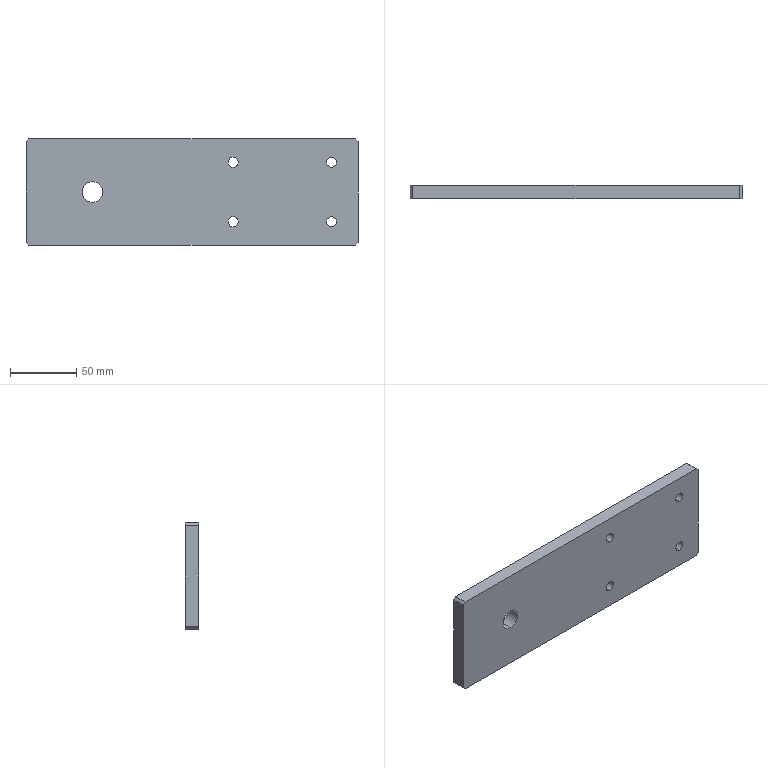Part | SolidWorks | features ICE 1, SplitBody 1 | 1 solid | 20 faces | box 250 x 10 x 80 mm | volume 196266 mm3 | cylinder 10 | plane 10 | commonest cylinder face diameters 7.5 x8 15.5 x2
STEP:
#1=CARTESIAN_POINT('',(-500.,-53.,-267.75));
#2=VERTEX_POINT('',#1);
#3=CARTESIAN_POINT('',(-500.,-53.,-252.25));
#4=VERTEX_POINT('',#3);
#5=CARTESIAN_POINT('',(-500.,-53.,-260.));
#6=DIRECTION('',(0.,-1.,0.));
#7=DIRECTION('',(0.,0.,-1.));
#8=AXIS2_PLACEMENT_3D('',#5,#6,#7);
#9=CIRCLE('',#8,7.75);
#10=EDGE_CURVE('',#2,#4,#9,.T.);
#11=ORIENTED_EDGE('',*,*,#10,.F.);
#12=CARTESIAN_POINT('',(-500.,-63.,-267.75));
#13=VERTEX_POINT('',#12);
#14=CARTESIAN_POINT('',(-500.,-58.,-267.75));
#15=DIRECTION('',(0.,-1.,0.));
#16=VECTOR('',#15,1000.);
#17=LINE('',#14,#16);
#18=EDGE_CURVE('',#2,#13,#17,.T.);
#19=ORIENTED_EDGE('',*,*,#18,.T.);
#20=CARTESIAN_POINT('',(-500.,-63.,-252.25));
#21=VERTEX_POINT('',#20);
#22=CARTESIAN_POINT('',(-500.,-63.,-260.));
#23=DIRECTION('',(0.,1.,0.));
#24=DIRECTION('',(0.,0.,1.));
#25=AXIS2_PLACEMENT_3D('',#22,#23,#24);
#26=CIRCLE('',#25,7.75);
#27=EDGE_CURVE('',#21,#13,#26,.T.);
#28=ORIENTED_EDGE('',*,*,#27,.F.);
#29=CARTESIAN_POINT('',(-500.,-58.,-252.25));
#30=DIRECTION('',(0.,-1.,0.));
#31=VECTOR('',#30,1000.);
#32=LINE('',#29,#31);
#33=EDGE_CURVE('',#4,#21,#32,.T.);
#34=ORIENTED_EDGE('',*,*,#33,.F.);
#35=EDGE_LOOP('',(#11,#19,#28,#34));
#36=FACE_OUTER_BOUND('',#35,.T.);
#37=CARTESIAN_POINT('',(-500.,-58.,-260.));
#38=DIRECTION('',(0.,-1.,0.));
#39=DIRECTION('',(0.,0.,1.));
#40=AXIS2_PLACEMENT_3D('',#37,#38,#39);
#41=CYLINDRICAL_SURFACE('',#40,7.75);
#42=ADVANCED_FACE('',(#36),#41,.F.);
#43=CARTESIAN_POINT('',(-394.,-53.,-241.35));
#44=VERTEX_POINT('',#43);
#45=CARTESIAN_POINT('',(-394.,-53.,-233.85));
#46=VERTEX_POINT('',#45);
#47=CARTESIAN_POINT('',(-394.,-53.,-237.6));
#48=DIRECTION('',(0.,-1.,0.));
#49=DIRECTION('',(0.,0.,-1.));
#50=AXIS2_PLACEMENT_3D('',#47,#48,#49);
#51=CIRCLE('',#50,3.75);
#52=EDGE_CURVE('',#44,#46,#51,.T.);
#53=ORIENTED_EDGE('',*,*,#52,.F.);
#54=CARTESIAN_POINT('',(-394.,-63.,-241.35));
#55=VERTEX_POINT('',#54);
#56=CARTESIAN_POINT('',(-394.,-58.,-241.35));
#57=DIRECTION('',(0.,-1.,0.));
#58=VECTOR('',#57,1000.);
#59=LINE('',#56,#58);
#60=EDGE_CURVE('',#44,#55,#59,.T.);
#61=ORIENTED_EDGE('',*,*,#60,.T.);
#62=CARTESIAN_POINT('',(-394.,-63.,-233.85));
#63=VERTEX_POINT('',#62);
#64=CARTESIAN_POINT('',(-394.,-63.,-237.6));
#65=DIRECTION('',(0.,1.,0.));
#66=DIRECTION('',(0.,0.,1.));
#67=AXIS2_PLACEMENT_3D('',#64,#65,#66);
#68=CIRCLE('',#67,3.75);
#69=EDGE_CURVE('',#63,#55,#68,.T.);
#70=ORIENTED_EDGE('',*,*,#69,.F.);
#71=CARTESIAN_POINT('',(-394.,-58.,-233.85));
#72=DIRECTION('',(0.,-1.,0.));
#73=VECTOR('',#72,1000.);
#74=LINE('',#71,#73);
#75=EDGE_CURVE('',#46,#63,#74,.T.);
#76=ORIENTED_EDGE('',*,*,#75,.F.);
#77=EDGE_LOOP('',(#53,#61,#70,#76));
#78=FACE_OUTER_BOUND('',#77,.T.);
#79=CARTESIAN_POINT('',(-394.,-58.,-237.6));
#80=DIRECTION('',(0.,-1.,0.));
#81=DIRECTION('',(0.,0.,1.));
#82=AXIS2_PLACEMENT_3D('',#79,#80,#81);
#83=CYLINDRICAL_SURFACE('',#82,3.75);
#84=ADVANCED_FACE('',(#78),#83,.F.);
#85=CARTESIAN_POINT('',(-320.,-53.,-241.35));
#86=VERTEX_POINT('',#85);
#87=CARTESIAN_POINT('',(-320.,-53.,-233.85));
#88=VERTEX_POINT('',#87);
#89=CARTESIAN_POINT('',(-320.,-53.,-237.6));
#90=DIRECTION('',(0.,-1.,0.));
#91=DIRECTION('',(0.,0.,-1.));
#92=AXIS2_PLACEMENT_3D('',#89,#90,#91);
#93=CIRCLE('',#92,3.75);
#94=EDGE_CURVE('',#86,#88,#93,.T.);
#95=ORIENTED_EDGE('',*,*,#94,.F.);
#96=CARTESIAN_POINT('',(-320.,-63.,-241.35));
#97=VERTEX_POINT('',#96);
#98=CARTESIAN_POINT('',(-320.,-58.,-241.35));
#99=DIRECTION('',(0.,-1.,0.));
#100=VECTOR('',#99,1000.);
#101=LINE('',#98,#100);
#102=EDGE_CURVE('',#86,#97,#101,.T.);
#103=ORIENTED_EDGE('',*,*,#102,.T.);
#104=CARTESIAN_POINT('',(-320.,-63.,-233.85));
#105=VERTEX_POINT('',#104);
#106=CARTESIAN_POINT('',(-320.,-63.,-237.6));
#107=DIRECTION('',(0.,1.,0.));
#108=DIRECTION('',(0.,0.,1.));
#109=AXIS2_PLACEMENT_3D('',#106,#107,#108);
#110=CIRCLE('',#109,3.75);
#111=EDGE_CURVE('',#105,#97,#110,.T.);
#112=ORIENTED_EDGE('',*,*,#111,.F.);
#113=CARTESIAN_POINT('',(-320.,-58.,-233.85));
#114=DIRECTION('',(0.,-1.,0.));
#115=VECTOR('',#114,1000.);
#116=LINE('',#113,#115);
#117=EDGE_CURVE('',#88,#105,#116,.T.);
#118=ORIENTED_EDGE('',*,*,#117,.F.);
#119=EDGE_LOOP('',(#95,#103,#112,#118));
#120=FACE_OUTER_BOUND('',#119,.T.);
#121=CARTESIAN_POINT('',(-320.,-58.,-237.6));
#122=DIRECTION('',(0.,-1.,0.));
#123=DIRECTION('',(0.,0.,1.));
#124=AXIS2_PLACEMENT_3D('',#121,#122,#123);
#125=CYLINDRICAL_SURFACE('',#124,3.75);
#126=ADVANCED_FACE('',(#120),#125,.F.);
#127=CARTESIAN_POINT('',(-320.,-53.,-286.15));
#128=VERTEX_POINT('',#127);
#129=CARTESIAN_POINT('',(-320.,-53.,-278.65));
#130=VERTEX_POINT('',#129);
#131=CARTESIAN_POINT('',(-320.,-53.,-282.4));
#132=DIRECTION('',(0.,-1.,0.));
#133=DIRECTION('',(0.,0.,-1.));
#134=AXIS2_PLACEMENT_3D('',#131,#132,#133);
#135=CIRCLE('',#134,3.75);
#136=EDGE_CURVE('',#128,#130,#135,.T.);
#137=ORIENTED_EDGE('',*,*,#136,.F.);
#138=CARTESIAN_POINT('',(-320.,-63.,-286.15));
#139=VERTEX_POINT('',#138);
#140=CARTESIAN_POINT('',(-320.,-58.,-286.15));
#141=DIRECTION('',(0.,-1.,0.));
#142=VECTOR('',#141,1000.);
#143=LINE('',#140,#142);
#144=EDGE_CURVE('',#128,#139,#143,.T.);
#145=ORIENTED_EDGE('',*,*,#144,.T.);
#146=CARTESIAN_POINT('',(-320.,-63.,-278.65));
#147=VERTEX_POINT('',#146);
#148=CARTESIAN_POINT('',(-320.,-63.,-282.4));
#149=DIRECTION('',(0.,1.,0.));
#150=DIRECTION('',(0.,0.,1.));
#151=AXIS2_PLACEMENT_3D('',#148,#149,#150);
#152=CIRCLE('',#151,3.75);
#153=EDGE_CURVE('',#147,#139,#152,.T.);
#154=ORIENTED_EDGE('',*,*,#153,.F.);
#155=CARTESIAN_POINT('',(-320.,-58.,-278.65));
#156=DIRECTION('',(0.,-1.,0.));
#157=VECTOR('',#156,1000.);
#158=LINE('',#155,#157);
#159=EDGE_CURVE('',#130,#147,#158,.T.);
#160=ORIENTED_EDGE('',*,*,#159,.F.);
#161=EDGE_LOOP('',(#137,#145,#154,#160));
#162=FACE_OUTER_BOUND('',#161,.T.);
#163=CARTESIAN_POINT('',(-320.,-58.,-282.4));
#164=DIRECTION('',(0.,-1.,0.));
#165=DIRECTION('',(0.,0.,1.));
#166=AXIS2_PLACEMENT_3D('',#163,#164,#165);
#167=CYLINDRICAL_SURFACE('',#166,3.75);
#168=ADVANCED_FACE('',(#162),#167,.F.);
#169=CARTESIAN_POINT('',(-394.,-53.,-286.15));
#170=VERTEX_POINT('',#169);
#171=CARTESIAN_POINT('',(-394.,-53.,-278.65));
#172=VERTEX_POINT('',#171);
#173=CARTESIAN_POINT('',(-394.,-53.,-282.4));
#174=DIRECTION('',(0.,-1.,0.));
#175=DIRECTION('',(0.,0.,-1.));
#176=AXIS2_PLACEMENT_3D('',#173,#174,#175);
#177=CIRCLE('',#176,3.75);
#178=EDGE_CURVE('',#170,#172,#177,.T.);
#179=ORIENTED_EDGE('',*,*,#178,.F.);
#180=CARTESIAN_POINT('',(-394.,-63.,-286.15));
#181=VERTEX_POINT('',#180);
#182=CARTESIAN_POINT('',(-394.,-58.,-286.15));
#183=DIRECTION('',(0.,-1.,0.));
#184=VECTOR('',#183,1000.);
#185=LINE('',#182,#184);
#186=EDGE_CURVE('',#170,#181,#185,.T.);
#187=ORIENTED_EDGE('',*,*,#186,.T.);
#188=CARTESIAN_POINT('',(-394.,-63.,-278.65));
#189=VERTEX_POINT('',#188);
#190=CARTESIAN_POINT('',(-394.,-63.,-282.4));
#191=DIRECTION('',(0.,1.,0.));
#192=DIRECTION('',(0.,0.,1.));
#193=AXIS2_PLACEMENT_3D('',#190,#191,#192);
#194=CIRCLE('',#193,3.75);
#195=EDGE_CURVE('',#189,#181,#194,.T.);
#196=ORIENTED_EDGE('',*,*,#195,.F.);
#197=CARTESIAN_POINT('',(-394.,-58.,-278.65));
#198=DIRECTION('',(0.,-1.,0.));
#199=VECTOR('',#198,1000.);
#200=LINE('',#197,#199);
#201=EDGE_CURVE('',#172,#189,#200,.T.);
#202=ORIENTED_EDGE('',*,*,#201,.F.);
#203=EDGE_LOOP('',(#179,#187,#196,#202));
#204=FACE_OUTER_BOUND('',#203,.T.);
#205=CARTESIAN_POINT('',(-394.,-58.,-282.4));
#206=DIRECTION('',(0.,-1.,0.));
#207=DIRECTION('',(0.,0.,1.));
#208=AXIS2_PLACEMENT_3D('',#205,#206,#207);
#209=CYLINDRICAL_SURFACE('',#208,3.75);
#210=ADVANCED_FACE('',(#204),#209,.F.);
#211=CARTESIAN_POINT('',(-550.,-53.,-298.));
#212=VERTEX_POINT('',#211);
#213=CARTESIAN_POINT('',(-550.,-53.,-222.));
#214=VERTEX_POINT('',#213);
#215=CARTESIAN_POINT('',(-550.,-53.,-300.));
#216=DIRECTION('',(0.,0.,1.));
#217=VECTOR('',#216,1000.);
#218=LINE('',#215,#217);
#219=EDGE_CURVE('',#212,#214,#218,.T.);
#220=ORIENTED_EDGE('',*,*,#219,.F.);
#221=CARTESIAN_POINT('',(-550.,-63.,-298.));
#222=VERTEX_POINT('',#221);
#223=CARTESIAN_POINT('',(-550.,-63.,-298.));
#224=DIRECTION('',(0.,1.,0.));
#225=VECTOR('',#224,1000.);
#226=LINE('',#223,#225);
#227=EDGE_CURVE('',#222,#212,#226,.T.);
#228=ORIENTED_EDGE('',*,*,#227,.F.);
#229=CARTESIAN_POINT('',(-550.,-63.,-222.));
#230=VERTEX_POINT('',#229);
#231=CARTESIAN_POINT('',(-550.,-63.,-300.));
#232=DIRECTION('',(0.,0.,1.));
#233=VECTOR('',#232,1000.);
#234=LINE('',#231,#233);
#235=EDGE_CURVE('',#222,#230,#234,.T.);
#236=ORIENTED_EDGE('',*,*,#235,.T.);
#237=CARTESIAN_POINT('',(-550.,-63.,-222.));
#238=DIRECTION('',(0.,-1.,0.));
#239=VECTOR('',#238,1000.);
#240=LINE('',#237,#239);
#241=EDGE_CURVE('',#214,#230,#240,.T.);
#242=ORIENTED_EDGE('',*,*,#241,.F.);
#243=EDGE_LOOP('',(#220,#228,#236,#242));
#244=FACE_OUTER_BOUND('',#243,.T.);
#245=CARTESIAN_POINT('',(-550.,-63.,-300.));
#246=DIRECTION('',(1.,0.,0.));
#247=DIRECTION('',(0.,1.,0.));
#248=AXIS2_PLACEMENT_3D('',#245,#246,#247);
#249=PLANE('',#248);
#250=ADVANCED_FACE('',(#244),#249,.F.);
#251=CARTESIAN_POINT('',(-548.,-53.,-220.));
#252=VERTEX_POINT('',#251);
#253=CARTESIAN_POINT('',(-302.,-53.,-220.));
#254=VERTEX_POINT('',#253);
#255=CARTESIAN_POINT('',(-550.,-53.,-220.));
#256=DIRECTION('',(1.,0.,0.));
#257=VECTOR('',#256,1000.);
#258=LINE('',#255,#257);
#259=EDGE_CURVE('',#252,#254,#258,.T.);
#260=ORIENTED_EDGE('',*,*,#259,.F.);
#261=CARTESIAN_POINT('',(-548.,-63.,-220.));
#262=VERTEX_POINT('',#261);
#263=CARTESIAN_POINT('',(-548.,-63.,-220.));
#264=DIRECTION('',(0.,1.,0.));
#265=VECTOR('',#264,1000.);
#266=LINE('',#263,#265);
#267=EDGE_CURVE('',#262,#252,#266,.T.);
#268=ORIENTED_EDGE('',*,*,#267,.F.);
#269=CARTESIAN_POINT('',(-302.,-63.,-220.));
#270=VERTEX_POINT('',#269);
#271=CARTESIAN_POINT('',(-550.,-63.,-220.));
#272=DIRECTION('',(1.,0.,0.));
#273=VECTOR('',#272,1000.);
#274=LINE('',#271,#273);
#275=EDGE_CURVE('',#262,#270,#274,.T.);
#276=ORIENTED_EDGE('',*,*,#275,.T.);
#277=CARTESIAN_POINT('',(-302.,-63.,-220.));
#278=DIRECTION('',(0.,-1.,0.));
#279=VECTOR('',#278,1000.);
#280=LINE('',#277,#279);
#281=EDGE_CURVE('',#254,#270,#280,.T.);
#282=ORIENTED_EDGE('',*,*,#281,.F.);
#283=EDGE_LOOP('',(#260,#268,#276,#282));
#284=FACE_OUTER_BOUND('',#283,.T.);
#285=CARTESIAN_POINT('',(-550.,-63.,-220.));
#286=DIRECTION('',(0.,0.,-1.));
#287=DIRECTION('',(0.,-1.,0.));
#288=AXIS2_PLACEMENT_3D('',#285,#286,#287);
#289=PLANE('',#288);
#290=ADVANCED_FACE('',(#284),#289,.F.);
#291=CARTESIAN_POINT('',(-300.,-63.,-222.));
#292=VERTEX_POINT('',#291);
#293=CARTESIAN_POINT('',(-300.,-63.,-298.));
#294=VERTEX_POINT('',#293);
#295=CARTESIAN_POINT('',(-300.,-63.,-300.));
#296=DIRECTION('',(0.,0.,-1.));
#297=VECTOR('',#296,1000.);
#298=LINE('',#295,#297);
#299=EDGE_CURVE('',#292,#294,#298,.T.);
#300=ORIENTED_EDGE('',*,*,#299,.T.);
#301=CARTESIAN_POINT('',(-300.,-53.,-298.));
#302=VERTEX_POINT('',#301);
#303=CARTESIAN_POINT('',(-300.,-63.,-298.));
#304=DIRECTION('',(0.,-1.,0.));
#305=VECTOR('',#304,1000.);
#306=LINE('',#303,#305);
#307=EDGE_CURVE('',#302,#294,#306,.T.);
#308=ORIENTED_EDGE('',*,*,#307,.F.);
#309=CARTESIAN_POINT('',(-300.,-53.,-222.));
#310=VERTEX_POINT('',#309);
#311=CARTESIAN_POINT('',(-300.,-53.,-300.));
#312=DIRECTION('',(0.,0.,-1.));
#313=VECTOR('',#312,1000.);
#314=LINE('',#311,#313);
#315=EDGE_CURVE('',#310,#302,#314,.T.);
#316=ORIENTED_EDGE('',*,*,#315,.F.);
#317=CARTESIAN_POINT('',(-300.,-63.,-222.));
#318=DIRECTION('',(0.,1.,0.));
#319=VECTOR('',#318,1000.);
#320=LINE('',#317,#319);
#321=EDGE_CURVE('',#292,#310,#320,.T.);
#322=ORIENTED_EDGE('',*,*,#321,.F.);
#323=EDGE_LOOP('',(#300,#308,#316,#322));
#324=FACE_OUTER_BOUND('',#323,.T.);
#325=CARTESIAN_POINT('',(-300.,-63.,-300.));
#326=DIRECTION('',(-1.,0.,0.));
#327=DIRECTION('',(0.,-1.,0.));
#328=AXIS2_PLACEMENT_3D('',#325,#326,#327);
#329=PLANE('',#328);
#330=ADVANCED_FACE('',(#324),#329,.F.);
#331=CARTESIAN_POINT('',(-302.,-63.,-300.));
#332=VERTEX_POINT('',#331);
#333=CARTESIAN_POINT('',(-548.,-63.,-300.));
#334=VERTEX_POINT('',#333);
#335=CARTESIAN_POINT('',(-550.,-63.,-300.));
#336=DIRECTION('',(-1.,0.,0.));
#337=VECTOR('',#336,1000.);
#338=LINE('',#335,#337);
#339=EDGE_CURVE('',#332,#334,#338,.T.);
#340=ORIENTED_EDGE('',*,*,#339,.T.);
#341=CARTESIAN_POINT('',(-548.,-53.,-300.));
#342=VERTEX_POINT('',#341);
#343=CARTESIAN_POINT('',(-548.,-63.,-300.));
#344=DIRECTION('',(0.,-1.,0.));
#345=VECTOR('',#344,1000.);
#346=LINE('',#343,#345);
#347=EDGE_CURVE('',#342,#334,#346,.T.);
#348=ORIENTED_EDGE('',*,*,#347,.F.);
#349=CARTESIAN_POINT('',(-302.,-53.,-300.));
#350=VERTEX_POINT('',#349);
#351=CARTESIAN_POINT('',(-550.,-53.,-300.));
#352=DIRECTION('',(-1.,0.,0.));
#353=VECTOR('',#352,1000.);
#354=LINE('',#351,#353);
#355=EDGE_CURVE('',#350,#342,#354,.T.);
#356=ORIENTED_EDGE('',*,*,#355,.F.);
#357=CARTESIAN_POINT('',(-302.,-63.,-300.));
#358=DIRECTION('',(0.,1.,0.));
#359=VECTOR('',#358,1000.);
#360=LINE('',#357,#359);
#361=EDGE_CURVE('',#332,#350,#360,.T.);
#362=ORIENTED_EDGE('',*,*,#361,.F.);
#363=EDGE_LOOP('',(#340,#348,#356,#362));
#364=FACE_OUTER_BOUND('',#363,.T.);
#365=CARTESIAN_POINT('',(-550.,-63.,-300.));
#366=DIRECTION('',(0.,0.,1.));
#367=DIRECTION('',(0.,1.,0.));
#368=AXIS2_PLACEMENT_3D('',#365,#366,#367);
#369=PLANE('',#368);
#370=ADVANCED_FACE('',(#364),#369,.F.);
#371=ORIENTED_EDGE('',*,*,#27,.T.);
#372=CARTESIAN_POINT('',(-500.,-63.,-260.));
#373=DIRECTION('',(0.,1.,0.));
#374=DIRECTION('',(0.,0.,1.));
#375=AXIS2_PLACEMENT_3D('',#372,#373,#374);
#376=CIRCLE('',#375,7.75);
#377=EDGE_CURVE('',#13,#21,#376,.T.);
#378=ORIENTED_EDGE('',*,*,#377,.T.);
#379=EDGE_LOOP('',(#371,#378));
#380=FACE_BOUND('',#379,.T.);
#381=ORIENTED_EDGE('',*,*,#69,.T.);
#382=CARTESIAN_POINT('',(-394.,-63.,-237.6));
#383=DIRECTION('',(0.,1.,0.));
#384=DIRECTION('',(0.,0.,1.));
#385=AXIS2_PLACEMENT_3D('',#382,#383,#384);
#386=CIRCLE('',#385,3.75);
#387=EDGE_CURVE('',#55,#63,#386,.T.);
#388=ORIENTED_EDGE('',*,*,#387,.T.);
#389=EDGE_LOOP('',(#381,#388));
#390=FACE_BOUND('',#389,.T.);
#391=ORIENTED_EDGE('',*,*,#111,.T.);
#392=CARTESIAN_POINT('',(-320.,-63.,-237.6));
#393=DIRECTION('',(0.,1.,0.));
#394=DIRECTION('',(0.,0.,1.));
#395=AXIS2_PLACEMENT_3D('',#392,#393,#394);
#396=CIRCLE('',#395,3.75);
#397=EDGE_CURVE('',#97,#105,#396,.T.);
#398=ORIENTED_EDGE('',*,*,#397,.T.);
#399=EDGE_LOOP('',(#391,#398));
#400=FACE_BOUND('',#399,.T.);
#401=ORIENTED_EDGE('',*,*,#153,.T.);
#402=CARTESIAN_POINT('',(-320.,-63.,-282.4));
#403=DIRECTION('',(0.,1.,0.));
#404=DIRECTION('',(0.,0.,1.));
#405=AXIS2_PLACEMENT_3D('',#402,#403,#404);
#406=CIRCLE('',#405,3.75);
#407=EDGE_CURVE('',#139,#147,#406,.T.);
#408=ORIENTED_EDGE('',*,*,#407,.T.);
#409=EDGE_LOOP('',(#401,#408));
#410=FACE_BOUND('',#409,.T.);
#411=ORIENTED_EDGE('',*,*,#195,.T.);
#412=CARTESIAN_POINT('',(-394.,-63.,-282.4));
#413=DIRECTION('',(0.,1.,0.));
#414=DIRECTION('',(0.,0.,1.));
#415=AXIS2_PLACEMENT_3D('',#412,#413,#414);
#416=CIRCLE('',#415,3.75);
#417=EDGE_CURVE('',#181,#189,#416,.T.);
#418=ORIENTED_EDGE('',*,*,#417,.T.);
#419=EDGE_LOOP('',(#411,#418));
#420=FACE_BOUND('',#419,.T.);
#421=ORIENTED_EDGE('',*,*,#275,.F.);
#422=CARTESIAN_POINT('',(-164.,-63.,164.));
#423=DIRECTION('',(0.7071,0.,0.7071));
#424=VECTOR('',#423,1000.);
#425=LINE('',#422,#424);
#426=EDGE_CURVE('',#230,#262,#425,.T.);
#427=ORIENTED_EDGE('',*,*,#426,.F.);
#428=ORIENTED_EDGE('',*,*,#235,.F.);
#429=CARTESIAN_POINT('',(-424.,-63.,-424.));
#430=DIRECTION('',(-0.7071,0.,0.7071));
#431=VECTOR('',#430,1000.);
#432=LINE('',#429,#431);
#433=EDGE_CURVE('',#334,#222,#432,.T.);
#434=ORIENTED_EDGE('',*,*,#433,.F.);
#435=ORIENTED_EDGE('',*,*,#339,.F.);
#436=CARTESIAN_POINT('',(-1.,-63.,1.));
#437=DIRECTION('',(-0.7071,0.,-0.7071));
#438=VECTOR('',#437,1000.);
#439=LINE('',#436,#438);
#440=EDGE_CURVE('',#294,#332,#439,.T.);
#441=ORIENTED_EDGE('',*,*,#440,.F.);
#442=ORIENTED_EDGE('',*,*,#299,.F.);
#443=CARTESIAN_POINT('',(-261.,-63.,-261.));
#444=DIRECTION('',(0.7071,0.,-0.7071));
#445=VECTOR('',#444,1000.);
#446=LINE('',#443,#445);
#447=EDGE_CURVE('',#270,#292,#446,.T.);
#448=ORIENTED_EDGE('',*,*,#447,.F.);
#449=EDGE_LOOP('',(#421,#427,#428,#434,#435,#441,#442,#448));
#450=FACE_OUTER_BOUND('',#449,.T.);
#451=CARTESIAN_POINT('',(0.,-63.,0.));
#452=DIRECTION('',(0.,-1.,0.));
#453=DIRECTION('',(0.,0.,1.));
#454=AXIS2_PLACEMENT_3D('',#451,#452,#453);
#455=PLANE('',#454);
#456=ADVANCED_FACE('',(#380,#390,#400,#410,#420,#450),#455,.T.);
#457=CARTESIAN_POINT('',(-394.,-53.,-237.6));
#458=DIRECTION('',(0.,-1.,0.));
#459=DIRECTION('',(0.,0.,-1.));
#460=AXIS2_PLACEMENT_3D('',#457,#458,#459);
#461=CIRCLE('',#460,3.75);
#462=EDGE_CURVE('',#46,#44,#461,.T.);
#463=ORIENTED_EDGE('',*,*,#462,.T.);
#464=ORIENTED_EDGE('',*,*,#52,.T.);
#465=EDGE_LOOP('',(#463,#464));
#466=FACE_BOUND('',#465,.T.);
#467=CARTESIAN_POINT('',(-394.,-53.,-282.4));
#468=DIRECTION('',(0.,-1.,0.));
#469=DIRECTION('',(0.,0.,-1.));
#470=AXIS2_PLACEMENT_3D('',#467,#468,#469);
#471=CIRCLE('',#470,3.75);
#472=EDGE_CURVE('',#172,#170,#471,.T.);
#473=ORIENTED_EDGE('',*,*,#472,.T.);
#474=ORIENTED_EDGE('',*,*,#178,.T.);
#475=EDGE_LOOP('',(#473,#474));
#476=FACE_BOUND('',#475,.T.);
#477=CARTESIAN_POINT('',(-320.,-53.,-237.6));
#478=DIRECTION('',(0.,-1.,0.));
#479=DIRECTION('',(0.,0.,-1.));
#480=AXIS2_PLACEMENT_3D('',#477,#478,#479);
#481=CIRCLE('',#480,3.75);
#482=EDGE_CURVE('',#88,#86,#481,.T.);
#483=ORIENTED_EDGE('',*,*,#482,.T.);
#484=ORIENTED_EDGE('',*,*,#94,.T.);
#485=EDGE_LOOP('',(#483,#484));
#486=FACE_BOUND('',#485,.T.);
#487=CARTESIAN_POINT('',(-320.,-53.,-282.4));
#488=DIRECTION('',(0.,-1.,0.));
#489=DIRECTION('',(0.,0.,-1.));
#490=AXIS2_PLACEMENT_3D('',#487,#488,#489);
#491=CIRCLE('',#490,3.75);
#492=EDGE_CURVE('',#130,#128,#491,.T.);
#493=ORIENTED_EDGE('',*,*,#492,.T.);
#494=ORIENTED_EDGE('',*,*,#136,.T.);
#495=EDGE_LOOP('',(#493,#494));
#496=FACE_BOUND('',#495,.T.);
#497=CARTESIAN_POINT('',(-500.,-53.,-260.));
#498=DIRECTION('',(0.,-1.,0.));
#499=DIRECTION('',(0.,0.,-1.));
#500=AXIS2_PLACEMENT_3D('',#497,#498,#499);
#501=CIRCLE('',#500,7.75);
#502=EDGE_CURVE('',#4,#2,#501,.T.);
#503=ORIENTED_EDGE('',*,*,#502,.T.);
#504=ORIENTED_EDGE('',*,*,#10,.T.);
#505=EDGE_LOOP('',(#503,#504));
#506=FACE_BOUND('',#505,.T.);
#507=ORIENTED_EDGE('',*,*,#315,.T.);
#508=CARTESIAN_POINT('',(-302.,-53.,-300.));
#509=DIRECTION('',(0.7071,0.,0.7071));
#510=VECTOR('',#509,1000.);
#511=LINE('',#508,#510);
#512=EDGE_CURVE('',#350,#302,#511,.T.);
#513=ORIENTED_EDGE('',*,*,#512,.F.);
#514=ORIENTED_EDGE('',*,*,#355,.T.);
#515=CARTESIAN_POINT('',(-550.,-53.,-298.));
#516=DIRECTION('',(0.7071,0.,-0.7071));
#517=VECTOR('',#516,1000.);
#518=LINE('',#515,#517);
#519=EDGE_CURVE('',#212,#342,#518,.T.);
#520=ORIENTED_EDGE('',*,*,#519,.F.);
#521=ORIENTED_EDGE('',*,*,#219,.T.);
#522=CARTESIAN_POINT('',(-548.,-53.,-220.));
#523=DIRECTION('',(-0.7071,0.,-0.7071));
#524=VECTOR('',#523,1000.);
#525=LINE('',#522,#524);
#526=EDGE_CURVE('',#252,#214,#525,.T.);
#527=ORIENTED_EDGE('',*,*,#526,.F.);
#528=ORIENTED_EDGE('',*,*,#259,.T.);
#529=CARTESIAN_POINT('',(-300.,-53.,-222.));
#530=DIRECTION('',(-0.7071,0.,0.7071));
#531=VECTOR('',#530,1000.);
#532=LINE('',#529,#531);
#533=EDGE_CURVE('',#310,#254,#532,.T.);
#534=ORIENTED_EDGE('',*,*,#533,.F.);
#535=EDGE_LOOP('',(#507,#513,#514,#520,#521,#527,#528,#534));
#536=FACE_OUTER_BOUND('',#535,.T.);
#537=CARTESIAN_POINT('',(0.,-53.,0.));
#538=DIRECTION('',(0.,-1.,0.));
#539=DIRECTION('',(0.,0.,1.));
#540=AXIS2_PLACEMENT_3D('',#537,#538,#539);
#541=PLANE('',#540);
#542=ADVANCED_FACE('',(#466,#476,#486,#496,#506,#536),#541,.F.);
#543=ORIENTED_EDGE('',*,*,#186,.F.);
#544=ORIENTED_EDGE('',*,*,#472,.F.);
#545=ORIENTED_EDGE('',*,*,#201,.T.);
#546=ORIENTED_EDGE('',*,*,#417,.F.);
#547=EDGE_LOOP('',(#543,#544,#545,#546));
#548=FACE_OUTER_BOUND('',#547,.T.);
#549=CARTESIAN_POINT('',(-394.,-58.,-282.4));
#550=DIRECTION('',(0.,-1.,0.));
#551=DIRECTION('',(0.,0.,1.));
#552=AXIS2_PLACEMENT_3D('',#549,#550,#551);
#553=CYLINDRICAL_SURFACE('',#552,3.75);
#554=ADVANCED_FACE('',(#548),#553,.F.);
#555=ORIENTED_EDGE('',*,*,#144,.F.);
#556=ORIENTED_EDGE('',*,*,#492,.F.);
#557=ORIENTED_EDGE('',*,*,#159,.T.);
#558=ORIENTED_EDGE('',*,*,#407,.F.);
#559=EDGE_LOOP('',(#555,#556,#557,#558));
#560=FACE_OUTER_BOUND('',#559,.T.);
#561=CARTESIAN_POINT('',(-320.,-58.,-282.4));
#562=DIRECTION('',(0.,-1.,0.));
#563=DIRECTION('',(0.,0.,1.));
#564=AXIS2_PLACEMENT_3D('',#561,#562,#563);
#565=CYLINDRICAL_SURFACE('',#564,3.75);
#566=ADVANCED_FACE('',(#560),#565,.F.);
#567=ORIENTED_EDGE('',*,*,#102,.F.);
#568=ORIENTED_EDGE('',*,*,#482,.F.);
#569=ORIENTED_EDGE('',*,*,#117,.T.);
#570=ORIENTED_EDGE('',*,*,#397,.F.);
#571=EDGE_LOOP('',(#567,#568,#569,#570));
#572=FACE_OUTER_BOUND('',#571,.T.);
#573=CARTESIAN_POINT('',(-320.,-58.,-237.6));
#574=DIRECTION('',(0.,-1.,0.));
#575=DIRECTION('',(0.,0.,1.));
#576=AXIS2_PLACEMENT_3D('',#573,#574,#575);
#577=CYLINDRICAL_SURFACE('',#576,3.75);
#578=ADVANCED_FACE('',(#572),#577,.F.);
#579=ORIENTED_EDGE('',*,*,#60,.F.);
#580=ORIENTED_EDGE('',*,*,#462,.F.);
#581=ORIENTED_EDGE('',*,*,#75,.T.);
#582=ORIENTED_EDGE('',*,*,#387,.F.);
#583=EDGE_LOOP('',(#579,#580,#581,#582));
#584=FACE_OUTER_BOUND('',#583,.T.);
#585=CARTESIAN_POINT('',(-394.,-58.,-237.6));
#586=DIRECTION('',(0.,-1.,0.));
#587=DIRECTION('',(0.,0.,1.));
#588=AXIS2_PLACEMENT_3D('',#585,#586,#587);
#589=CYLINDRICAL_SURFACE('',#588,3.75);
#590=ADVANCED_FACE('',(#584),#589,.F.);
#591=ORIENTED_EDGE('',*,*,#447,.T.);
#592=ORIENTED_EDGE('',*,*,#321,.T.);
#593=ORIENTED_EDGE('',*,*,#533,.T.);
#594=ORIENTED_EDGE('',*,*,#281,.T.);
#595=EDGE_LOOP('',(#591,#592,#593,#594));
#596=FACE_OUTER_BOUND('',#595,.T.);
#597=CARTESIAN_POINT('',(-300.,-63.,-222.));
#598=DIRECTION('',(-0.7071,0.,-0.7071));
#599=DIRECTION('',(0.,1.,0.));
#600=AXIS2_PLACEMENT_3D('',#597,#598,#599);
#601=PLANE('',#600);
#602=ADVANCED_FACE('',(#596),#601,.F.);
#603=ORIENTED_EDGE('',*,*,#440,.T.);
#604=ORIENTED_EDGE('',*,*,#361,.T.);
#605=ORIENTED_EDGE('',*,*,#512,.T.);
#606=ORIENTED_EDGE('',*,*,#307,.T.);
#607=EDGE_LOOP('',(#603,#604,#605,#606));
#608=FACE_OUTER_BOUND('',#607,.T.);
#609=CARTESIAN_POINT('',(-302.,-63.,-300.));
#610=DIRECTION('',(-0.7071,0.,0.7071));
#611=DIRECTION('',(0.,1.,0.));
#612=AXIS2_PLACEMENT_3D('',#609,#610,#611);
#613=PLANE('',#612);
#614=ADVANCED_FACE('',(#608),#613,.F.);
#615=ORIENTED_EDGE('',*,*,#426,.T.);
#616=ORIENTED_EDGE('',*,*,#267,.T.);
#617=ORIENTED_EDGE('',*,*,#526,.T.);
#618=ORIENTED_EDGE('',*,*,#241,.T.);
#619=EDGE_LOOP('',(#615,#616,#617,#618));
#620=FACE_OUTER_BOUND('',#619,.T.);
#621=CARTESIAN_POINT('',(-548.,-63.,-220.));
#622=DIRECTION('',(0.7071,0.,-0.7071));
#623=DIRECTION('',(0.,1.,0.));
#624=AXIS2_PLACEMENT_3D('',#621,#622,#623);
#625=PLANE('',#624);
#626=ADVANCED_FACE('',(#620),#625,.F.);
#627=ORIENTED_EDGE('',*,*,#433,.T.);
#628=ORIENTED_EDGE('',*,*,#227,.T.);
#629=ORIENTED_EDGE('',*,*,#519,.T.);
#630=ORIENTED_EDGE('',*,*,#347,.T.);
#631=EDGE_LOOP('',(#627,#628,#629,#630));
#632=FACE_OUTER_BOUND('',#631,.T.);
#633=CARTESIAN_POINT('',(-550.,-63.,-298.));
#634=DIRECTION('',(0.7071,0.,0.7071));
#635=DIRECTION('',(0.,1.,0.));
#636=AXIS2_PLACEMENT_3D('',#633,#634,#635);
#637=PLANE('',#636);
#638=ADVANCED_FACE('',(#632),#637,.F.);
#639=ORIENTED_EDGE('',*,*,#18,.F.);
#640=ORIENTED_EDGE('',*,*,#502,.F.);
#641=ORIENTED_EDGE('',*,*,#33,.T.);
#642=ORIENTED_EDGE('',*,*,#377,.F.);
#643=EDGE_LOOP('',(#639,#640,#641,#642));
#644=FACE_OUTER_BOUND('',#643,.T.);
#645=CARTESIAN_POINT('',(-500.,-58.,-260.));
#646=DIRECTION('',(0.,-1.,0.));
#647=DIRECTION('',(0.,0.,1.));
#648=AXIS2_PLACEMENT_3D('',#645,#646,#647);
#649=CYLINDRICAL_SURFACE('',#648,7.75);
#650=ADVANCED_FACE('',(#644),#649,.F.);
#651=CLOSED_SHELL('',(#42,#84,#126,#168,#210,#250,#290,#330,#370,#456,#542,#554,#566,#578,#590,#602,#614,#626,#638,#650));
#652=MANIFOLD_SOLID_BREP('',#651);
#653=CARTESIAN_POINT('',(0.,0.,0.));
#654=DIRECTION('',(0.,0.,1.));
#655=DIRECTION('',(1.,0.,0.));
#656=AXIS2_PLACEMENT_3D('',#653,#654,#655);
#657=(LENGTH_UNIT()NAMED_UNIT(*)SI_UNIT(.MILLI.,.METRE.));
#658=UNCERTAINTY_MEASURE_WITH_UNIT(LENGTH_MEASURE(0.00001),#657,'','');
#659=(NAMED_UNIT(*)PLANE_ANGLE_UNIT()SI_UNIT($,.RADIAN.));
#660=(NAMED_UNIT(*)SI_UNIT($,.STERADIAN.)SOLID_ANGLE_UNIT());
#661=(GEOMETRIC_REPRESENTATION_CONTEXT(3)GLOBAL_UNCERTAINTY_ASSIGNED_CONTEXT((#658))GLOBAL_UNIT_ASSIGNED_CONTEXT((#657,#659,#660))REPRESENTATION_CONTEXT('',''));
#662=ADVANCED_BREP_SHAPE_REPRESENTATION('',(#652,#656),#661);